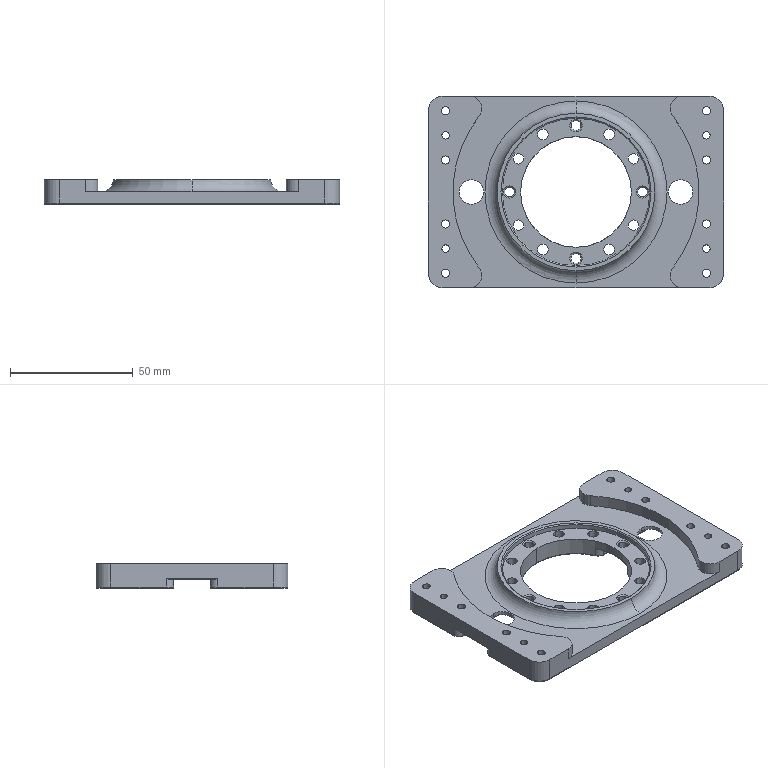Part | 1 solid | 226 faces | box 120 x 78 x 10 mm | volume 45562 mm3 | cylinder 134 | plane 47 | cone 26 | torus 19 | commonest cylinder face diameters 6 x24 3.3 x16 4 x16 4.3 x16 7.6 x16 1 x12